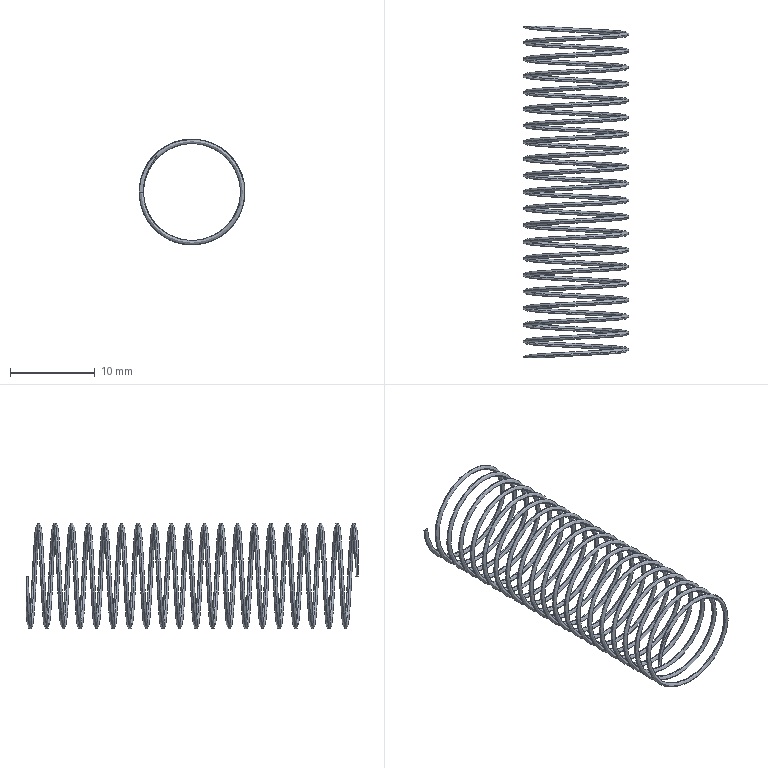Part | SolidWorks | features ICE 1, Sweep 1 | 1 solid | 6 faces | box 12.5 x 39.277 x 12.5 mm | volume 146.671 mm3 | plane 4 | spline 2